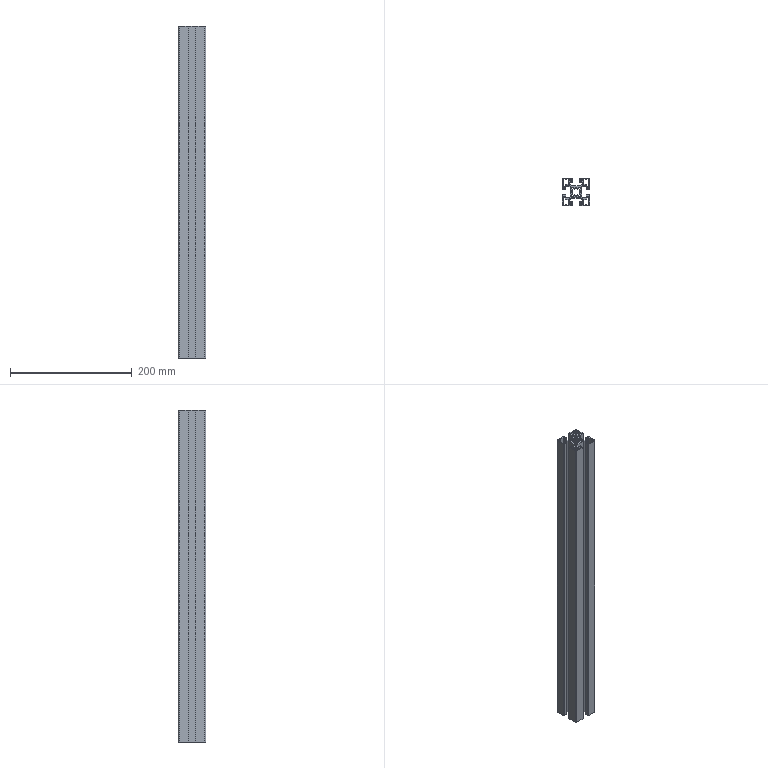Part | SolidWorks | features Extrusion 1 | 1 solid | 236 faces | box 45 x 45 x 545 mm | volume 347775 mm3 | plane 178 | cylinder 58 | commonest cylinder face diameters 2 x36 3 x10 12 x8 4 x4